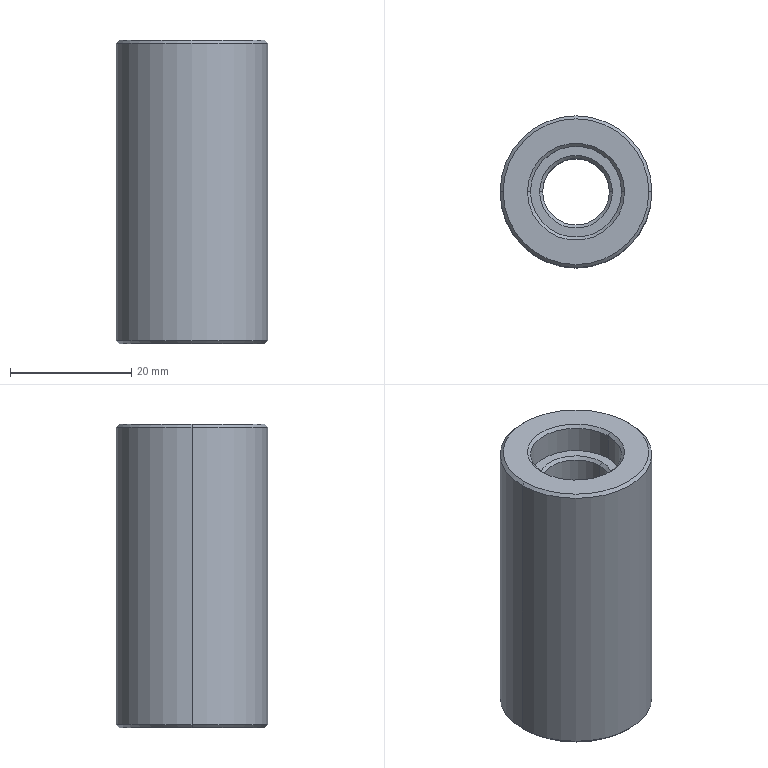Part | STEP file | 10000054363swp000-1 | 1 solid | 24 faces | box 25 x 25 x 50 mm | volume 18935 mm3 | cone 12 | cylinder 8 | plane 4 | commonest cylinder face diameters 15 x4 11 x2 25 x2
STEP:
#1=CARTESIAN_POINT('',(7.5,0.,-24.5));
#2=VERTEX_POINT('',#1);
#3=CARTESIAN_POINT('',(-7.5,0.,-24.5));
#4=VERTEX_POINT('',#3);
#5=CARTESIAN_POINT('',(0.,0.,-24.5));
#6=DIRECTION('',(0.,0.,-1.));
#7=DIRECTION('',(1.,0.,0.));
#8=AXIS2_PLACEMENT_3D('',#5,#6,#7);
#9=CIRCLE('',#8,7.5);
#10=EDGE_CURVE('',#2,#4,#9,.T.);
#11=ORIENTED_EDGE('',*,*,#10,.F.);
#12=CARTESIAN_POINT('',(8.,0.,-25.));
#13=VERTEX_POINT('',#12);
#14=CARTESIAN_POINT('',(7.5,0.,-24.5));
#15=DIRECTION('',(0.7071,0.,-0.7071));
#16=VECTOR('',#15,1000.);
#17=LINE('',#14,#16);
#18=EDGE_CURVE('',#2,#13,#17,.T.);
#19=ORIENTED_EDGE('',*,*,#18,.T.);
#20=CARTESIAN_POINT('',(-8.,0.,-25.));
#21=VERTEX_POINT('',#20);
#22=CARTESIAN_POINT('',(0.,0.,-25.));
#23=DIRECTION('',(0.,0.,1.));
#24=DIRECTION('',(1.,0.,0.));
#25=AXIS2_PLACEMENT_3D('',#22,#23,#24);
#26=CIRCLE('',#25,8.);
#27=EDGE_CURVE('',#21,#13,#26,.T.);
#28=ORIENTED_EDGE('',*,*,#27,.F.);
#29=CARTESIAN_POINT('',(-7.5,0.,-24.5));
#30=DIRECTION('',(-0.7071,0.,-0.7071));
#31=VECTOR('',#30,1000.);
#32=LINE('',#29,#31);
#33=EDGE_CURVE('',#4,#21,#32,.T.);
#34=ORIENTED_EDGE('',*,*,#33,.F.);
#35=EDGE_LOOP('',(#11,#19,#28,#34));
#36=FACE_OUTER_BOUND('',#35,.T.);
#37=CARTESIAN_POINT('',(0.,0.,-24.5));
#38=DIRECTION('',(0.,0.,-1.));
#39=DIRECTION('',(-1.,0.,0.));
#40=AXIS2_PLACEMENT_3D('',#37,#38,#39);
#41=CONICAL_SURFACE('',#40,7.5,0.7854);
#42=ADVANCED_FACE('',(#36),#41,.F.);
#43=CARTESIAN_POINT('',(-7.5,0.,24.5));
#44=VERTEX_POINT('',#43);
#45=CARTESIAN_POINT('',(7.5,0.,24.5));
#46=VERTEX_POINT('',#45);
#47=CARTESIAN_POINT('',(0.,0.,24.5));
#48=DIRECTION('',(0.,0.,1.));
#49=DIRECTION('',(1.,0.,0.));
#50=AXIS2_PLACEMENT_3D('',#47,#48,#49);
#51=CIRCLE('',#50,7.5);
#52=EDGE_CURVE('',#44,#46,#51,.T.);
#53=ORIENTED_EDGE('',*,*,#52,.F.);
#54=CARTESIAN_POINT('',(-8.,0.,25.));
#55=VERTEX_POINT('',#54);
#56=CARTESIAN_POINT('',(-7.5,0.,24.5));
#57=DIRECTION('',(-0.7071,0.,0.7071));
#58=VECTOR('',#57,1000.);
#59=LINE('',#56,#58);
#60=EDGE_CURVE('',#44,#55,#59,.T.);
#61=ORIENTED_EDGE('',*,*,#60,.T.);
#62=CARTESIAN_POINT('',(8.,0.,25.));
#63=VERTEX_POINT('',#62);
#64=CARTESIAN_POINT('',(0.,0.,25.));
#65=DIRECTION('',(0.,0.,-1.));
#66=DIRECTION('',(1.,0.,0.));
#67=AXIS2_PLACEMENT_3D('',#64,#65,#66);
#68=CIRCLE('',#67,8.);
#69=EDGE_CURVE('',#63,#55,#68,.T.);
#70=ORIENTED_EDGE('',*,*,#69,.F.);
#71=CARTESIAN_POINT('',(7.5,0.,24.5));
#72=DIRECTION('',(0.7071,0.,0.7071));
#73=VECTOR('',#72,1000.);
#74=LINE('',#71,#73);
#75=EDGE_CURVE('',#46,#63,#74,.T.);
#76=ORIENTED_EDGE('',*,*,#75,.F.);
#77=EDGE_LOOP('',(#53,#61,#70,#76));
#78=FACE_OUTER_BOUND('',#77,.T.);
#79=CARTESIAN_POINT('',(0.,0.,24.5));
#80=DIRECTION('',(0.,0.,1.));
#81=DIRECTION('',(1.,0.,0.));
#82=AXIS2_PLACEMENT_3D('',#79,#80,#81);
#83=CONICAL_SURFACE('',#82,7.5,0.7854);
#84=ADVANCED_FACE('',(#78),#83,.F.);
#85=CARTESIAN_POINT('',(12.,0.,25.));
#86=VERTEX_POINT('',#85);
#87=CARTESIAN_POINT('',(-12.,0.,25.));
#88=VERTEX_POINT('',#87);
#89=CARTESIAN_POINT('',(0.,0.,25.));
#90=DIRECTION('',(0.,0.,1.));
#91=DIRECTION('',(1.,0.,0.));
#92=AXIS2_PLACEMENT_3D('',#89,#90,#91);
#93=CIRCLE('',#92,12.);
#94=EDGE_CURVE('',#86,#88,#93,.T.);
#95=ORIENTED_EDGE('',*,*,#94,.F.);
#96=CARTESIAN_POINT('',(12.5,0.,24.5));
#97=VERTEX_POINT('',#96);
#98=CARTESIAN_POINT('',(12.,0.,25.));
#99=DIRECTION('',(0.7071,0.,-0.7071));
#100=VECTOR('',#99,1000.);
#101=LINE('',#98,#100);
#102=EDGE_CURVE('',#86,#97,#101,.T.);
#103=ORIENTED_EDGE('',*,*,#102,.T.);
#104=CARTESIAN_POINT('',(-12.5,0.,24.5));
#105=VERTEX_POINT('',#104);
#106=CARTESIAN_POINT('',(0.,0.,24.5));
#107=DIRECTION('',(0.,0.,-1.));
#108=DIRECTION('',(1.,0.,0.));
#109=AXIS2_PLACEMENT_3D('',#106,#107,#108);
#110=CIRCLE('',#109,12.5);
#111=EDGE_CURVE('',#105,#97,#110,.T.);
#112=ORIENTED_EDGE('',*,*,#111,.F.);
#113=CARTESIAN_POINT('',(-12.,0.,25.));
#114=DIRECTION('',(-0.7071,0.,-0.7071));
#115=VECTOR('',#114,1000.);
#116=LINE('',#113,#115);
#117=EDGE_CURVE('',#88,#105,#116,.T.);
#118=ORIENTED_EDGE('',*,*,#117,.F.);
#119=EDGE_LOOP('',(#95,#103,#112,#118));
#120=FACE_OUTER_BOUND('',#119,.T.);
#121=CARTESIAN_POINT('',(0.,0.,25.));
#122=DIRECTION('',(0.,0.,-1.));
#123=DIRECTION('',(-1.,0.,0.));
#124=AXIS2_PLACEMENT_3D('',#121,#122,#123);
#125=CONICAL_SURFACE('',#124,12.,0.7854);
#126=ADVANCED_FACE('',(#120),#125,.T.);
#127=CARTESIAN_POINT('',(-12.,0.,-25.));
#128=VERTEX_POINT('',#127);
#129=CARTESIAN_POINT('',(12.,0.,-25.));
#130=VERTEX_POINT('',#129);
#131=CARTESIAN_POINT('',(0.,0.,-25.));
#132=DIRECTION('',(0.,0.,-1.));
#133=DIRECTION('',(1.,0.,0.));
#134=AXIS2_PLACEMENT_3D('',#131,#132,#133);
#135=CIRCLE('',#134,12.);
#136=EDGE_CURVE('',#128,#130,#135,.T.);
#137=ORIENTED_EDGE('',*,*,#136,.F.);
#138=CARTESIAN_POINT('',(-12.5,0.,-24.5));
#139=VERTEX_POINT('',#138);
#140=CARTESIAN_POINT('',(-12.5,0.,-24.5));
#141=DIRECTION('',(-0.7071,0.,0.7071));
#142=VECTOR('',#141,1000.);
#143=LINE('',#140,#142);
#144=EDGE_CURVE('',#128,#139,#143,.T.);
#145=ORIENTED_EDGE('',*,*,#144,.T.);
#146=CARTESIAN_POINT('',(12.5,0.,-24.5));
#147=VERTEX_POINT('',#146);
#148=CARTESIAN_POINT('',(0.,0.,-24.5));
#149=DIRECTION('',(0.,0.,1.));
#150=DIRECTION('',(1.,0.,0.));
#151=AXIS2_PLACEMENT_3D('',#148,#149,#150);
#152=CIRCLE('',#151,12.5);
#153=EDGE_CURVE('',#147,#139,#152,.T.);
#154=ORIENTED_EDGE('',*,*,#153,.F.);
#155=CARTESIAN_POINT('',(12.5,0.,-24.5));
#156=DIRECTION('',(0.7071,0.,0.7071));
#157=VECTOR('',#156,1000.);
#158=LINE('',#155,#157);
#159=EDGE_CURVE('',#130,#147,#158,.T.);
#160=ORIENTED_EDGE('',*,*,#159,.F.);
#161=EDGE_LOOP('',(#137,#145,#154,#160));
#162=FACE_OUTER_BOUND('',#161,.T.);
#163=CARTESIAN_POINT('',(0.,0.,-24.5));
#164=DIRECTION('',(0.,0.,1.));
#165=DIRECTION('',(1.,0.,0.));
#166=AXIS2_PLACEMENT_3D('',#163,#164,#165);
#167=CONICAL_SURFACE('',#166,12.5,0.7854);
#168=ADVANCED_FACE('',(#162),#167,.T.);
#169=CARTESIAN_POINT('',(5.5,0.,-19.5));
#170=VERTEX_POINT('',#169);
#171=CARTESIAN_POINT('',(-5.5,0.,-19.5));
#172=VERTEX_POINT('',#171);
#173=CARTESIAN_POINT('',(0.,0.,-19.5));
#174=DIRECTION('',(0.,0.,-1.));
#175=DIRECTION('',(1.,0.,0.));
#176=AXIS2_PLACEMENT_3D('',#173,#174,#175);
#177=CIRCLE('',#176,5.5);
#178=EDGE_CURVE('',#170,#172,#177,.T.);
#179=ORIENTED_EDGE('',*,*,#178,.F.);
#180=CARTESIAN_POINT('',(6.,0.,-20.));
#181=VERTEX_POINT('',#180);
#182=CARTESIAN_POINT('',(6.,0.,-20.));
#183=DIRECTION('',(0.7071,0.,-0.7071));
#184=VECTOR('',#183,1000.);
#185=LINE('',#182,#184);
#186=EDGE_CURVE('',#170,#181,#185,.T.);
#187=ORIENTED_EDGE('',*,*,#186,.T.);
#188=CARTESIAN_POINT('',(-6.,0.,-20.));
#189=VERTEX_POINT('',#188);
#190=CARTESIAN_POINT('',(0.,0.,-20.));
#191=DIRECTION('',(0.,0.,1.));
#192=DIRECTION('',(1.,0.,0.));
#193=AXIS2_PLACEMENT_3D('',#190,#191,#192);
#194=CIRCLE('',#193,6.);
#195=EDGE_CURVE('',#189,#181,#194,.T.);
#196=ORIENTED_EDGE('',*,*,#195,.F.);
#197=CARTESIAN_POINT('',(-6.,0.,-20.));
#198=DIRECTION('',(-0.7071,0.,-0.7071));
#199=VECTOR('',#198,1000.);
#200=LINE('',#197,#199);
#201=EDGE_CURVE('',#172,#189,#200,.T.);
#202=ORIENTED_EDGE('',*,*,#201,.F.);
#203=EDGE_LOOP('',(#179,#187,#196,#202));
#204=FACE_OUTER_BOUND('',#203,.T.);
#205=CARTESIAN_POINT('',(0.,0.,-20.));
#206=DIRECTION('',(0.,0.,-1.));
#207=DIRECTION('',(-1.,0.,0.));
#208=AXIS2_PLACEMENT_3D('',#205,#206,#207);
#209=CONICAL_SURFACE('',#208,6.,0.7854);
#210=ADVANCED_FACE('',(#204),#209,.F.);
#211=CARTESIAN_POINT('',(-5.5,0.,19.5));
#212=VERTEX_POINT('',#211);
#213=CARTESIAN_POINT('',(5.5,0.,19.5));
#214=VERTEX_POINT('',#213);
#215=CARTESIAN_POINT('',(0.,0.,19.5));
#216=DIRECTION('',(0.,0.,1.));
#217=DIRECTION('',(-1.,0.,0.));
#218=AXIS2_PLACEMENT_3D('',#215,#216,#217);
#219=CIRCLE('',#218,5.5);
#220=EDGE_CURVE('',#212,#214,#219,.T.);
#221=ORIENTED_EDGE('',*,*,#220,.F.);
#222=CARTESIAN_POINT('',(-6.,0.,20.));
#223=VERTEX_POINT('',#222);
#224=CARTESIAN_POINT('',(-6.,0.,20.));
#225=DIRECTION('',(-0.7071,0.,0.7071));
#226=VECTOR('',#225,1000.);
#227=LINE('',#224,#226);
#228=EDGE_CURVE('',#212,#223,#227,.T.);
#229=ORIENTED_EDGE('',*,*,#228,.T.);
#230=CARTESIAN_POINT('',(6.,0.,20.));
#231=VERTEX_POINT('',#230);
#232=CARTESIAN_POINT('',(0.,0.,20.));
#233=DIRECTION('',(0.,0.,-1.));
#234=DIRECTION('',(-1.,0.,0.));
#235=AXIS2_PLACEMENT_3D('',#232,#233,#234);
#236=CIRCLE('',#235,6.);
#237=EDGE_CURVE('',#231,#223,#236,.T.);
#238=ORIENTED_EDGE('',*,*,#237,.F.);
#239=CARTESIAN_POINT('',(6.,0.,20.));
#240=DIRECTION('',(0.7071,0.,0.7071));
#241=VECTOR('',#240,1000.);
#242=LINE('',#239,#241);
#243=EDGE_CURVE('',#214,#231,#242,.T.);
#244=ORIENTED_EDGE('',*,*,#243,.F.);
#245=EDGE_LOOP('',(#221,#229,#238,#244));
#246=FACE_OUTER_BOUND('',#245,.T.);
#247=CARTESIAN_POINT('',(0.,0.,20.));
#248=DIRECTION('',(0.,0.,1.));
#249=DIRECTION('',(1.,0.,0.));
#250=AXIS2_PLACEMENT_3D('',#247,#248,#249);
#251=CONICAL_SURFACE('',#250,6.,0.7854);
#252=ADVANCED_FACE('',(#246),#251,.F.);
#253=CARTESIAN_POINT('',(7.5,0.,-20.));
#254=VERTEX_POINT('',#253);
#255=CARTESIAN_POINT('',(-7.5,0.,-20.));
#256=VERTEX_POINT('',#255);
#257=CARTESIAN_POINT('',(0.,0.,-20.));
#258=DIRECTION('',(0.,0.,-1.));
#259=DIRECTION('',(-1.,0.,0.));
#260=AXIS2_PLACEMENT_3D('',#257,#258,#259);
#261=CIRCLE('',#260,7.5);
#262=EDGE_CURVE('',#254,#256,#261,.T.);
#263=ORIENTED_EDGE('',*,*,#262,.F.);
#264=CARTESIAN_POINT('',(7.5,0.,-25.));
#265=DIRECTION('',(0.,0.,-1.));
#266=VECTOR('',#265,1000.);
#267=LINE('',#264,#266);
#268=EDGE_CURVE('',#254,#2,#267,.T.);
#269=ORIENTED_EDGE('',*,*,#268,.T.);
#270=ORIENTED_EDGE('',*,*,#10,.T.);
#271=CARTESIAN_POINT('',(-7.5,0.,-25.));
#272=DIRECTION('',(0.,0.,-1.));
#273=VECTOR('',#272,1000.);
#274=LINE('',#271,#273);
#275=EDGE_CURVE('',#256,#4,#274,.T.);
#276=ORIENTED_EDGE('',*,*,#275,.F.);
#277=EDGE_LOOP('',(#263,#269,#270,#276));
#278=FACE_OUTER_BOUND('',#277,.T.);
#279=CARTESIAN_POINT('',(0.,0.,-25.));
#280=DIRECTION('',(0.,0.,-1.));
#281=DIRECTION('',(-1.,0.,0.));
#282=AXIS2_PLACEMENT_3D('',#279,#280,#281);
#283=CYLINDRICAL_SURFACE('',#282,7.5);
#284=ADVANCED_FACE('',(#278),#283,.F.);
#285=CARTESIAN_POINT('',(-7.5,0.,20.));
#286=VERTEX_POINT('',#285);
#287=CARTESIAN_POINT('',(7.5,0.,20.));
#288=VERTEX_POINT('',#287);
#289=CARTESIAN_POINT('',(0.,0.,20.));
#290=DIRECTION('',(0.,0.,1.));
#291=DIRECTION('',(1.,0.,0.));
#292=AXIS2_PLACEMENT_3D('',#289,#290,#291);
#293=CIRCLE('',#292,7.5);
#294=EDGE_CURVE('',#286,#288,#293,.T.);
#295=ORIENTED_EDGE('',*,*,#294,.F.);
#296=CARTESIAN_POINT('',(-7.5,0.,25.));
#297=DIRECTION('',(0.,0.,1.));
#298=VECTOR('',#297,1000.);
#299=LINE('',#296,#298);
#300=EDGE_CURVE('',#286,#44,#299,.T.);
#301=ORIENTED_EDGE('',*,*,#300,.T.);
#302=ORIENTED_EDGE('',*,*,#52,.T.);
#303=CARTESIAN_POINT('',(7.5,0.,25.));
#304=DIRECTION('',(0.,0.,1.));
#305=VECTOR('',#304,1000.);
#306=LINE('',#303,#305);
#307=EDGE_CURVE('',#288,#46,#306,.T.);
#308=ORIENTED_EDGE('',*,*,#307,.F.);
#309=EDGE_LOOP('',(#295,#301,#302,#308));
#310=FACE_OUTER_BOUND('',#309,.T.);
#311=CARTESIAN_POINT('',(0.,0.,25.));
#312=DIRECTION('',(0.,0.,1.));
#313=DIRECTION('',(1.,0.,0.));
#314=AXIS2_PLACEMENT_3D('',#311,#312,#313);
#315=CYLINDRICAL_SURFACE('',#314,7.5);
#316=ADVANCED_FACE('',(#310),#315,.F.);
#317=ORIENTED_EDGE('',*,*,#220,.T.);
#318=CARTESIAN_POINT('',(5.5,0.,25.));
#319=DIRECTION('',(0.,0.,-1.));
#320=VECTOR('',#319,1000.);
#321=LINE('',#318,#320);
#322=EDGE_CURVE('',#214,#170,#321,.T.);
#323=ORIENTED_EDGE('',*,*,#322,.T.);
#324=ORIENTED_EDGE('',*,*,#178,.T.);
#325=CARTESIAN_POINT('',(-5.5,0.,25.));
#326=DIRECTION('',(0.,0.,-1.));
#327=VECTOR('',#326,1000.);
#328=LINE('',#325,#327);
#329=EDGE_CURVE('',#212,#172,#328,.T.);
#330=ORIENTED_EDGE('',*,*,#329,.F.);
#331=EDGE_LOOP('',(#317,#323,#324,#330));
#332=FACE_OUTER_BOUND('',#331,.T.);
#333=CARTESIAN_POINT('',(0.,0.,25.));
#334=DIRECTION('',(0.,0.,-1.));
#335=DIRECTION('',(-1.,0.,0.));
#336=AXIS2_PLACEMENT_3D('',#333,#334,#335);
#337=CYLINDRICAL_SURFACE('',#336,5.5);
#338=ADVANCED_FACE('',(#332),#337,.F.);
#339=ORIENTED_EDGE('',*,*,#111,.T.);
#340=CARTESIAN_POINT('',(12.5,0.,25.));
#341=DIRECTION('',(0.,0.,-1.));
#342=VECTOR('',#341,1000.);
#343=LINE('',#340,#342);
#344=EDGE_CURVE('',#97,#147,#343,.T.);
#345=ORIENTED_EDGE('',*,*,#344,.T.);
#346=ORIENTED_EDGE('',*,*,#153,.T.);
#347=CARTESIAN_POINT('',(-12.5,0.,25.));
#348=DIRECTION('',(0.,0.,-1.));
#349=VECTOR('',#348,1000.);
#350=LINE('',#347,#349);
#351=EDGE_CURVE('',#105,#139,#350,.T.);
#352=ORIENTED_EDGE('',*,*,#351,.F.);
#353=EDGE_LOOP('',(#339,#345,#346,#352));
#354=FACE_OUTER_BOUND('',#353,.T.);
#355=CARTESIAN_POINT('',(0.,0.,25.));
#356=DIRECTION('',(0.,0.,-1.));
#357=DIRECTION('',(-1.,0.,0.));
#358=AXIS2_PLACEMENT_3D('',#355,#356,#357);
#359=CYLINDRICAL_SURFACE('',#358,12.5);
#360=ADVANCED_FACE('',(#354),#359,.T.);
#361=CARTESIAN_POINT('',(0.,0.,25.));
#362=DIRECTION('',(0.,0.,1.));
#363=DIRECTION('',(1.,0.,0.));
#364=AXIS2_PLACEMENT_3D('',#361,#362,#363);
#365=CIRCLE('',#364,12.);
#366=EDGE_CURVE('',#88,#86,#365,.T.);
#367=ORIENTED_EDGE('',*,*,#366,.T.);
#368=ORIENTED_EDGE('',*,*,#94,.T.);
#369=EDGE_LOOP('',(#367,#368));
#370=FACE_OUTER_BOUND('',#369,.T.);
#371=ORIENTED_EDGE('',*,*,#69,.T.);
#372=CARTESIAN_POINT('',(0.,0.,25.));
#373=DIRECTION('',(0.,0.,-1.));
#374=DIRECTION('',(1.,0.,0.));
#375=AXIS2_PLACEMENT_3D('',#372,#373,#374);
#376=CIRCLE('',#375,8.);
#377=EDGE_CURVE('',#55,#63,#376,.T.);
#378=ORIENTED_EDGE('',*,*,#377,.T.);
#379=EDGE_LOOP('',(#371,#378));
#380=FACE_BOUND('',#379,.T.);
#381=CARTESIAN_POINT('',(0.,0.,25.));
#382=DIRECTION('',(0.,0.,1.));
#383=DIRECTION('',(1.,0.,0.));
#384=AXIS2_PLACEMENT_3D('',#381,#382,#383);
#385=PLANE('',#384);
#386=ADVANCED_FACE('',(#370,#380),#385,.T.);
#387=CARTESIAN_POINT('',(0.,0.,-25.));
#388=DIRECTION('',(0.,0.,-1.));
#389=DIRECTION('',(1.,0.,0.));
#390=AXIS2_PLACEMENT_3D('',#387,#388,#389);
#391=CIRCLE('',#390,12.);
#392=EDGE_CURVE('',#130,#128,#391,.T.);
#393=ORIENTED_EDGE('',*,*,#392,.T.);
#394=ORIENTED_EDGE('',*,*,#136,.T.);
#395=EDGE_LOOP('',(#393,#394));
#396=FACE_OUTER_BOUND('',#395,.T.);
#397=ORIENTED_EDGE('',*,*,#27,.T.);
#398=CARTESIAN_POINT('',(0.,0.,-25.));
#399=DIRECTION('',(0.,0.,1.));
#400=DIRECTION('',(1.,0.,0.));
#401=AXIS2_PLACEMENT_3D('',#398,#399,#400);
#402=CIRCLE('',#401,8.);
#403=EDGE_CURVE('',#13,#21,#402,.T.);
#404=ORIENTED_EDGE('',*,*,#403,.T.);
#405=EDGE_LOOP('',(#397,#404));
#406=FACE_BOUND('',#405,.T.);
#407=CARTESIAN_POINT('',(0.,0.,-25.));
#408=DIRECTION('',(0.,0.,1.));
#409=DIRECTION('',(1.,0.,0.));
#410=AXIS2_PLACEMENT_3D('',#407,#408,#409);
#411=PLANE('',#410);
#412=ADVANCED_FACE('',(#396,#406),#411,.F.);
#413=ORIENTED_EDGE('',*,*,#344,.F.);
#414=CARTESIAN_POINT('',(0.,0.,24.5));
#415=DIRECTION('',(0.,0.,-1.));
#416=DIRECTION('',(1.,0.,0.));
#417=AXIS2_PLACEMENT_3D('',#414,#415,#416);
#418=CIRCLE('',#417,12.5);
#419=EDGE_CURVE('',#97,#105,#418,.T.);
#420=ORIENTED_EDGE('',*,*,#419,.T.);
#421=ORIENTED_EDGE('',*,*,#351,.T.);
#422=CARTESIAN_POINT('',(0.,0.,-24.5));
#423=DIRECTION('',(0.,0.,1.));
#424=DIRECTION('',(1.,0.,0.));
#425=AXIS2_PLACEMENT_3D('',#422,#423,#424);
#426=CIRCLE('',#425,12.5);
#427=EDGE_CURVE('',#139,#147,#426,.T.);
#428=ORIENTED_EDGE('',*,*,#427,.T.);
#429=EDGE_LOOP('',(#413,#420,#421,#428));
#430=FACE_OUTER_BOUND('',#429,.T.);
#431=CARTESIAN_POINT('',(0.,0.,25.));
#432=DIRECTION('',(0.,0.,-1.));
#433=DIRECTION('',(-1.,0.,0.));
#434=AXIS2_PLACEMENT_3D('',#431,#432,#433);
#435=CYLINDRICAL_SURFACE('',#434,12.5);
#436=ADVANCED_FACE('',(#430),#435,.T.);
#437=ORIENTED_EDGE('',*,*,#322,.F.);
#438=CARTESIAN_POINT('',(0.,0.,19.5));
#439=DIRECTION('',(0.,0.,1.));
#440=DIRECTION('',(-1.,0.,0.));
#441=AXIS2_PLACEMENT_3D('',#438,#439,#440);
#442=CIRCLE('',#441,5.5);
#443=EDGE_CURVE('',#214,#212,#442,.T.);
#444=ORIENTED_EDGE('',*,*,#443,.T.);
#445=ORIENTED_EDGE('',*,*,#329,.T.);
#446=CARTESIAN_POINT('',(0.,0.,-19.5));
#447=DIRECTION('',(0.,0.,-1.));
#448=DIRECTION('',(1.,0.,0.));
#449=AXIS2_PLACEMENT_3D('',#446,#447,#448);
#450=CIRCLE('',#449,5.5);
#451=EDGE_CURVE('',#172,#170,#450,.T.);
#452=ORIENTED_EDGE('',*,*,#451,.T.);
#453=EDGE_LOOP('',(#437,#444,#445,#452));
#454=FACE_OUTER_BOUND('',#453,.T.);
#455=CARTESIAN_POINT('',(0.,0.,25.));
#456=DIRECTION('',(0.,0.,-1.));
#457=DIRECTION('',(-1.,0.,0.));
#458=AXIS2_PLACEMENT_3D('',#455,#456,#457);
#459=CYLINDRICAL_SURFACE('',#458,5.5);
#460=ADVANCED_FACE('',(#454),#459,.F.);
#461=ORIENTED_EDGE('',*,*,#237,.T.);
#462=CARTESIAN_POINT('',(0.,0.,20.));
#463=DIRECTION('',(0.,0.,-1.));
#464=DIRECTION('',(-1.,0.,0.));
#465=AXIS2_PLACEMENT_3D('',#462,#463,#464);
#466=CIRCLE('',#465,6.);
#467=EDGE_CURVE('',#223,#231,#466,.T.);
#468=ORIENTED_EDGE('',*,*,#467,.T.);
#469=EDGE_LOOP('',(#461,#468));
#470=FACE_BOUND('',#469,.T.);
#471=CARTESIAN_POINT('',(0.,0.,20.));
#472=DIRECTION('',(0.,0.,1.));
#473=DIRECTION('',(1.,0.,0.));
#474=AXIS2_PLACEMENT_3D('',#471,#472,#473);
#475=CIRCLE('',#474,7.5);
#476=EDGE_CURVE('',#288,#286,#475,.T.);
#477=ORIENTED_EDGE('',*,*,#476,.T.);
#478=ORIENTED_EDGE('',*,*,#294,.T.);
#479=EDGE_LOOP('',(#477,#478));
#480=FACE_OUTER_BOUND('',#479,.T.);
#481=CARTESIAN_POINT('',(0.,0.,20.));
#482=DIRECTION('',(0.,0.,-1.));
#483=DIRECTION('',(-1.,0.,0.));
#484=AXIS2_PLACEMENT_3D('',#481,#482,#483);
#485=PLANE('',#484);
#486=ADVANCED_FACE('',(#470,#480),#485,.F.);
#487=ORIENTED_EDGE('',*,*,#300,.F.);
#488=ORIENTED_EDGE('',*,*,#476,.F.);
#489=ORIENTED_EDGE('',*,*,#307,.T.);
#490=CARTESIAN_POINT('',(0.,0.,24.5));
#491=DIRECTION('',(0.,0.,1.));
#492=DIRECTION('',(1.,0.,0.));
#493=AXIS2_PLACEMENT_3D('',#490,#491,#492);
#494=CIRCLE('',#493,7.5);
#495=EDGE_CURVE('',#46,#44,#494,.T.);
#496=ORIENTED_EDGE('',*,*,#495,.T.);
#497=EDGE_LOOP('',(#487,#488,#489,#496));
#498=FACE_OUTER_BOUND('',#497,.T.);
#499=CARTESIAN_POINT('',(0.,0.,25.));
#500=DIRECTION('',(0.,0.,1.));
#501=DIRECTION('',(1.,0.,0.));
#502=AXIS2_PLACEMENT_3D('',#499,#500,#501);
#503=CYLINDRICAL_SURFACE('',#502,7.5);
#504=ADVANCED_FACE('',(#498),#503,.F.);
#505=ORIENTED_EDGE('',*,*,#195,.T.);
#506=CARTESIAN_POINT('',(0.,0.,-20.));
#507=DIRECTION('',(0.,0.,1.));
#508=DIRECTION('',(1.,0.,0.));
#509=AXIS2_PLACEMENT_3D('',#506,#507,#508);
#510=CIRCLE('',#509,6.);
#511=EDGE_CURVE('',#181,#189,#510,.T.);
#512=ORIENTED_EDGE('',*,*,#511,.T.);
#513=EDGE_LOOP('',(#505,#512));
#514=FACE_BOUND('',#513,.T.);
#515=CARTESIAN_POINT('',(0.,0.,-20.));
#516=DIRECTION('',(0.,0.,-1.));
#517=DIRECTION('',(-1.,0.,0.));
#518=AXIS2_PLACEMENT_3D('',#515,#516,#517);
#519=CIRCLE('',#518,7.5);
#520=EDGE_CURVE('',#256,#254,#519,.T.);
#521=ORIENTED_EDGE('',*,*,#520,.T.);
#522=ORIENTED_EDGE('',*,*,#262,.T.);
#523=EDGE_LOOP('',(#521,#522));
#524=FACE_OUTER_BOUND('',#523,.T.);
#525=CARTESIAN_POINT('',(0.,0.,-20.));
#526=DIRECTION('',(0.,0.,1.));
#527=DIRECTION('',(1.,0.,0.));
#528=AXIS2_PLACEMENT_3D('',#525,#526,#527);
#529=PLANE('',#528);
#530=ADVANCED_FACE('',(#514,#524),#529,.F.);
#531=ORIENTED_EDGE('',*,*,#268,.F.);
#532=ORIENTED_EDGE('',*,*,#520,.F.);
#533=ORIENTED_EDGE('',*,*,#275,.T.);
#534=CARTESIAN_POINT('',(0.,0.,-24.5));
#535=DIRECTION('',(0.,0.,-1.));
#536=DIRECTION('',(1.,0.,0.));
#537=AXIS2_PLACEMENT_3D('',#534,#535,#536);
#538=CIRCLE('',#537,7.5);
#539=EDGE_CURVE('',#4,#2,#538,.T.);
#540=ORIENTED_EDGE('',*,*,#539,.T.);
#541=EDGE_LOOP('',(#531,#532,#533,#540));
#542=FACE_OUTER_BOUND('',#541,.T.);
#543=CARTESIAN_POINT('',(0.,0.,-25.));
#544=DIRECTION('',(0.,0.,-1.));
#545=DIRECTION('',(-1.,0.,0.));
#546=AXIS2_PLACEMENT_3D('',#543,#544,#545);
#547=CYLINDRICAL_SURFACE('',#546,7.5);
#548=ADVANCED_FACE('',(#542),#547,.F.);
#549=ORIENTED_EDGE('',*,*,#228,.F.);
#550=ORIENTED_EDGE('',*,*,#443,.F.);
#551=ORIENTED_EDGE('',*,*,#243,.T.);
#552=ORIENTED_EDGE('',*,*,#467,.F.);
#553=EDGE_LOOP('',(#549,#550,#551,#552));
#554=FACE_OUTER_BOUND('',#553,.T.);
#555=CARTESIAN_POINT('',(0.,0.,20.));
#556=DIRECTION('',(0.,0.,1.));
#557=DIRECTION('',(1.,0.,0.));
#558=AXIS2_PLACEMENT_3D('',#555,#556,#557);
#559=CONICAL_SURFACE('',#558,6.,0.7854);
#560=ADVANCED_FACE('',(#554),#559,.F.);
#561=ORIENTED_EDGE('',*,*,#186,.F.);
#562=ORIENTED_EDGE('',*,*,#451,.F.);
#563=ORIENTED_EDGE('',*,*,#201,.T.);
#564=ORIENTED_EDGE('',*,*,#511,.F.);
#565=EDGE_LOOP('',(#561,#562,#563,#564));
#566=FACE_OUTER_BOUND('',#565,.T.);
#567=CARTESIAN_POINT('',(0.,0.,-20.));
#568=DIRECTION('',(0.,0.,-1.));
#569=DIRECTION('',(-1.,0.,0.));
#570=AXIS2_PLACEMENT_3D('',#567,#568,#569);
#571=CONICAL_SURFACE('',#570,6.,0.7854);
#572=ADVANCED_FACE('',(#566),#571,.F.);
#573=ORIENTED_EDGE('',*,*,#144,.F.);
#574=ORIENTED_EDGE('',*,*,#392,.F.);
#575=ORIENTED_EDGE('',*,*,#159,.T.);
#576=ORIENTED_EDGE('',*,*,#427,.F.);
#577=EDGE_LOOP('',(#573,#574,#575,#576));
#578=FACE_OUTER_BOUND('',#577,.T.);
#579=CARTESIAN_POINT('',(0.,0.,-24.5));
#580=DIRECTION('',(0.,0.,1.));
#581=DIRECTION('',(1.,0.,0.));
#582=AXIS2_PLACEMENT_3D('',#579,#580,#581);
#583=CONICAL_SURFACE('',#582,12.5,0.7854);
#584=ADVANCED_FACE('',(#578),#583,.T.);
#585=ORIENTED_EDGE('',*,*,#102,.F.);
#586=ORIENTED_EDGE('',*,*,#366,.F.);
#587=ORIENTED_EDGE('',*,*,#117,.T.);
#588=ORIENTED_EDGE('',*,*,#419,.F.);
#589=EDGE_LOOP('',(#585,#586,#587,#588));
#590=FACE_OUTER_BOUND('',#589,.T.);
#591=CARTESIAN_POINT('',(0.,0.,25.));
#592=DIRECTION('',(0.,0.,-1.));
#593=DIRECTION('',(-1.,0.,0.));
#594=AXIS2_PLACEMENT_3D('',#591,#592,#593);
#595=CONICAL_SURFACE('',#594,12.,0.7854);
#596=ADVANCED_FACE('',(#590),#595,.T.);
#597=ORIENTED_EDGE('',*,*,#60,.F.);
#598=ORIENTED_EDGE('',*,*,#495,.F.);
#599=ORIENTED_EDGE('',*,*,#75,.T.);
#600=ORIENTED_EDGE('',*,*,#377,.F.);
#601=EDGE_LOOP('',(#597,#598,#599,#600));
#602=FACE_OUTER_BOUND('',#601,.T.);
#603=CARTESIAN_POINT('',(0.,0.,24.5));
#604=DIRECTION('',(0.,0.,1.));
#605=DIRECTION('',(1.,0.,0.));
#606=AXIS2_PLACEMENT_3D('',#603,#604,#605);
#607=CONICAL_SURFACE('',#606,7.5,0.7854);
#608=ADVANCED_FACE('',(#602),#607,.F.);
#609=ORIENTED_EDGE('',*,*,#18,.F.);
#610=ORIENTED_EDGE('',*,*,#539,.F.);
#611=ORIENTED_EDGE('',*,*,#33,.T.);
#612=ORIENTED_EDGE('',*,*,#403,.F.);
#613=EDGE_LOOP('',(#609,#610,#611,#612));
#614=FACE_OUTER_BOUND('',#613,.T.);
#615=CARTESIAN_POINT('',(0.,0.,-24.5));
#616=DIRECTION('',(0.,0.,-1.));
#617=DIRECTION('',(-1.,0.,0.));
#618=AXIS2_PLACEMENT_3D('',#615,#616,#617);
#619=CONICAL_SURFACE('',#618,7.5,0.7854);
#620=ADVANCED_FACE('',(#614),#619,.F.);
#621=CLOSED_SHELL('',(#42,#84,#126,#168,#210,#252,#284,#316,#338,#360,#386,#412,#436,#460,#486,#504,#530,#548,#560,#572,#584,#596,#608,#620));
#622=MANIFOLD_SOLID_BREP('',#621);
#623=CARTESIAN_POINT('',(0.,0.,0.));
#624=DIRECTION('',(0.,0.,1.));
#625=DIRECTION('',(1.,0.,0.));
#626=AXIS2_PLACEMENT_3D('',#623,#624,#625);
#627=(LENGTH_UNIT()NAMED_UNIT(*)SI_UNIT(.MILLI.,.METRE.));
#628=UNCERTAINTY_MEASURE_WITH_UNIT(LENGTH_MEASURE(0.00001),#627,'','');
#629=(NAMED_UNIT(*)PLANE_ANGLE_UNIT()SI_UNIT($,.RADIAN.));
#630=(NAMED_UNIT(*)SI_UNIT($,.STERADIAN.)SOLID_ANGLE_UNIT());
#631=(GEOMETRIC_REPRESENTATION_CONTEXT(3)GLOBAL_UNCERTAINTY_ASSIGNED_CONTEXT((#628))GLOBAL_UNIT_ASSIGNED_CONTEXT((#627,#629,#630))REPRESENTATION_CONTEXT('',''));
#632=ADVANCED_BREP_SHAPE_REPRESENTATION('',(#622,#626),#631);